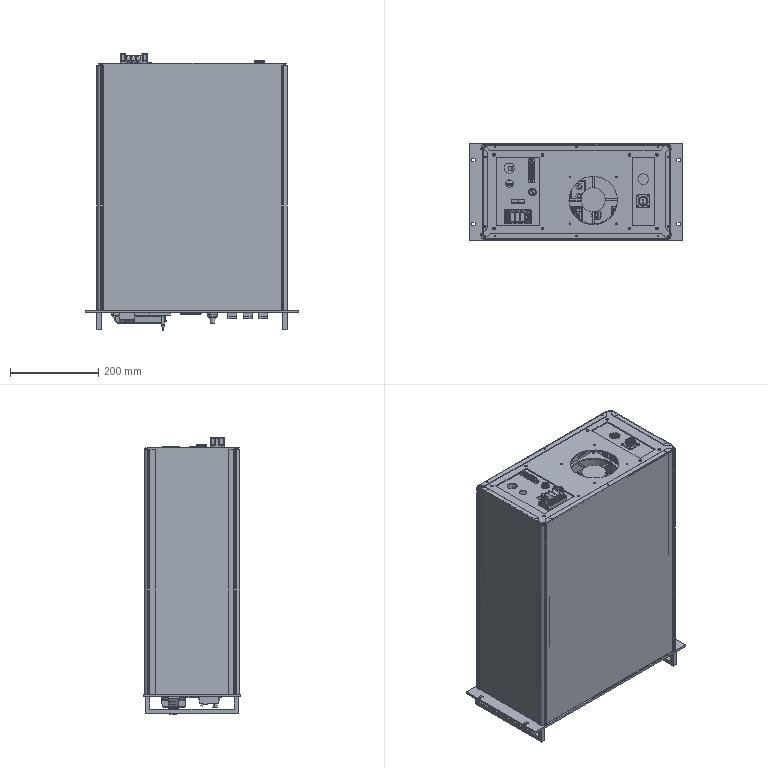Part | SolidWorks | features BaseBody 45 | 45 solids | 4258 faces | volume 4228574 mm3 | plane 2713 | cylinder 1234 | spline 175 | torus 74 | cone 52 | sphere 10 | commonest cylinder face diameters 3 x374 2.5 x134 3.3 x68 4 x59 1.5 x50 6.5 x43